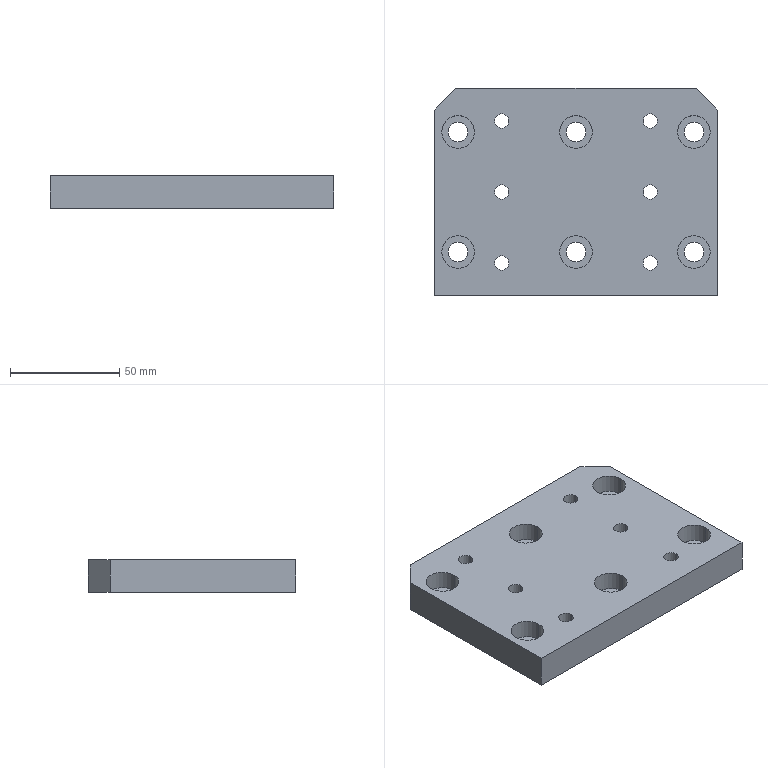Part | SolidWorks | features HoleWzd 2, Chamfer 1, Extrusion 1 | 1 solid | 68 faces | box 130 x 95 x 15 mm | volume 166774 mm3 | cylinder 48 | plane 20 | commonest cylinder face diameters 6.6 x12 9 x12 11 x12 15 x12